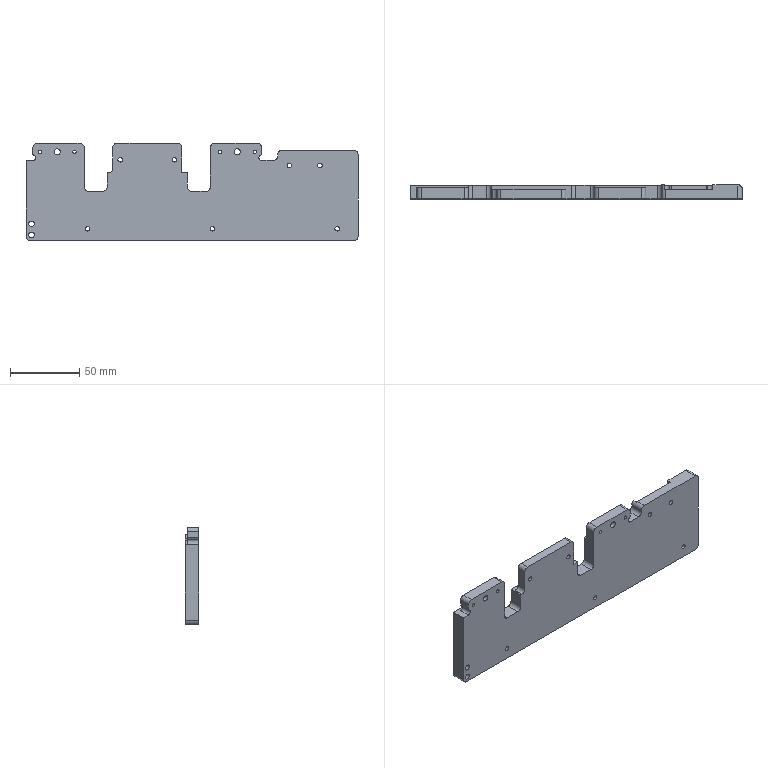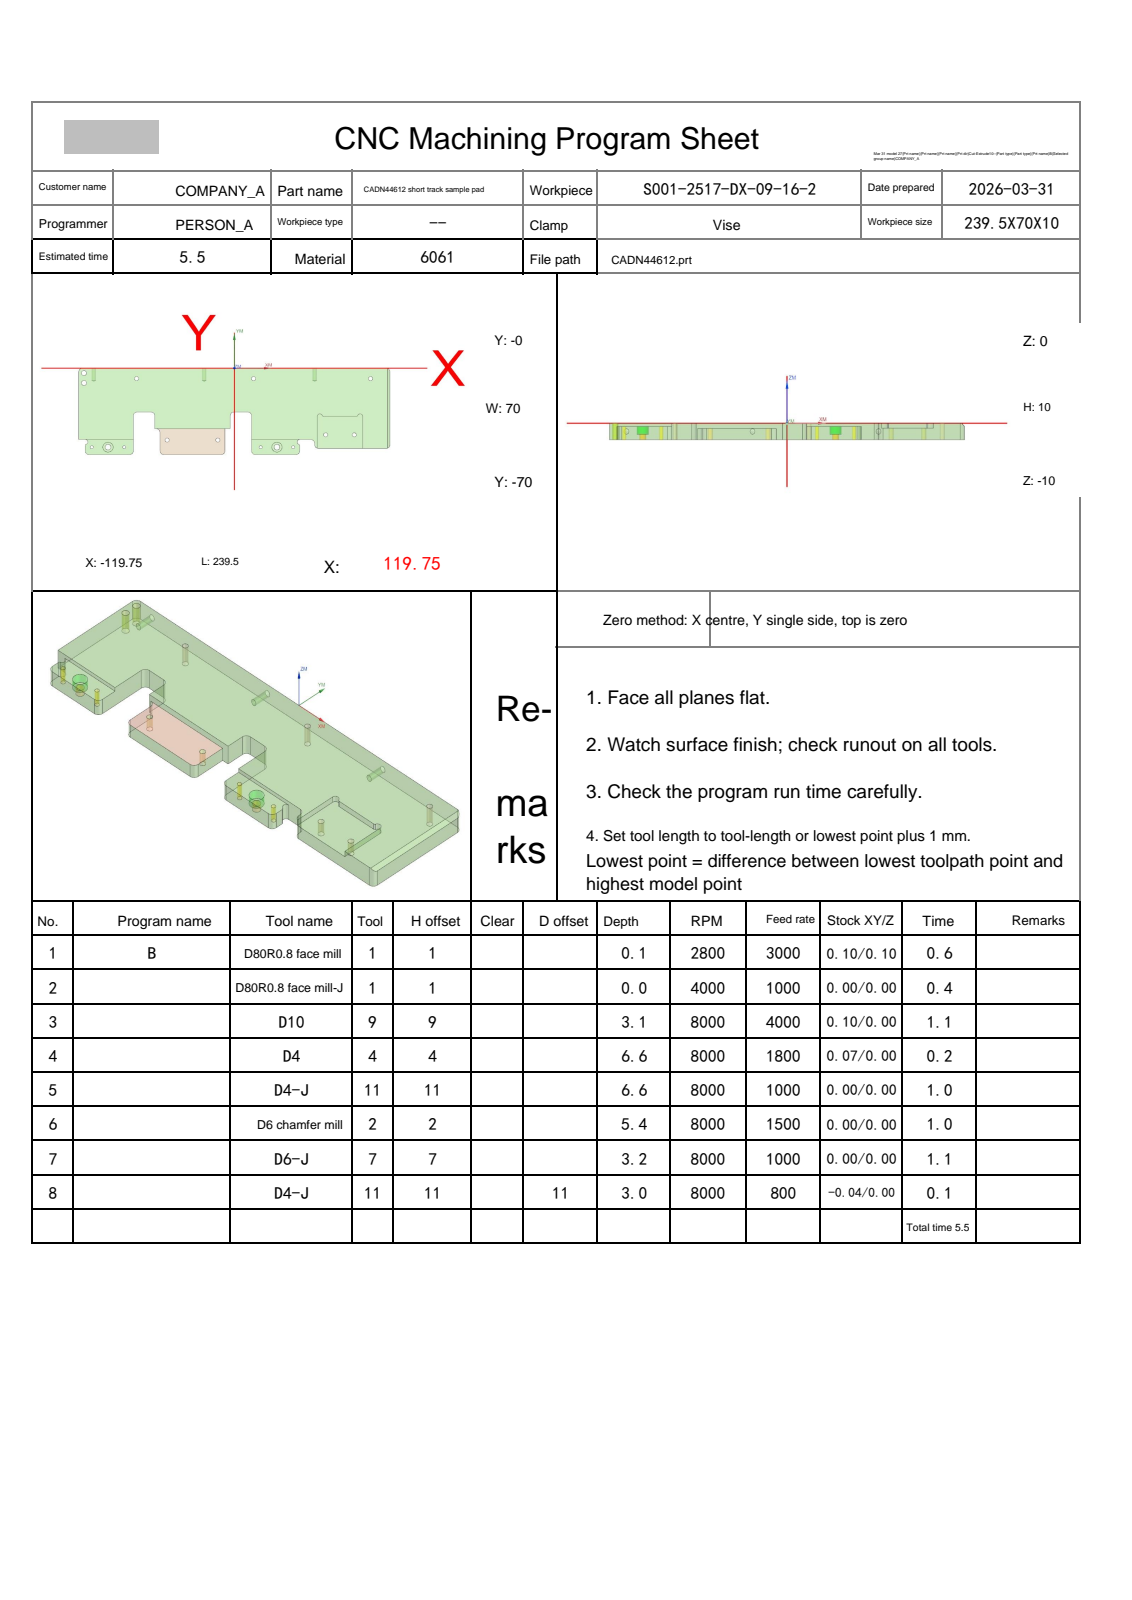NC program | NX | posted by the shop | part box 239.5 x 10 x 70 mm
Whole program, first 1746 of 1845 lines:
%
O0001
(Machine time: 7.06 MIN)
(===Total Tool:6===)
(T1=D80R0.8 face mill D=80.  R=0.8  D-  H01 Z=0.    )
(T9=D10     D=10.  R=0.   D-  H09 Z=-3.1  )
(T4=D4      D=4.   R=0.   D-  H04 Z=-6.6  )
(T11=D4-J   D=4.   R=0.   D-  H11 Z=-6.6  )
(T2=D6 chamfer mill   D=6.   R=0.   D-  H02 Z=-5.4  )
(T7=D6-J    D=6.   R=0.   D7  H07 Z=-3.2  )
G80 G90 G17 G49 G40
G91 G28 Z0
M01
N1 T01 M06
(D80R0.8 face mill  D=80. R=0.8 H=01 ce=0.10 di=0.10)
G00 G90 G54 X-171.847 Y-37.679 M03 S2800
G43 H01 Z20.
M08
Z3.525
G01 Z1.525 F3000.
X-159.847 Y-37.445
X159.847 Y-31.197
X171.847 Y-30.963
Z3.525
G00 X-171.847 Y-37.679
Z3.05
G01 Z1.05
X-159.847 Y-37.445
X159.847 Y-31.197
X171.847 Y-30.963
Z3.05
G00 X-171.847 Y-37.679
Z2.575
G01 Z.575
X-159.847 Y-37.445
X159.847 Y-31.197
X171.847 Y-30.963
Z2.575
G00 X-171.847 Y-37.679
Z2.1
G01 Z.1
X-159.847 Y-37.445
X159.847 Y-31.197
X171.847 Y-30.963
Z2.1
G00 Z20.
G91 G28 Z0.0
M05
M09
G91 G28 Z0.0
M01
N2 T01 M06
(D80R0.8 face mill-J  D=80. R=0.8 H=01 ce=0.00 di=0.00)
G00 G90 G54 X-171.749 Y-37.674 M03 S4000
G43 H01 Z20.
M08
Z2.
G01 Z0.0 F1000.
X-159.749 Y-37.44
X159.749 Y-31.203
X171.749 Y-30.969
Z2.
G00 Z20.
G91 G28 Z0.0
M05
M09
G91 G28 Z0.0
M01
N3 T09 M06
(D10  D=10. R=0. H=09 ce=0.10 di=0.10)
G00 G90 G54 X-122.211 Y-70.4 M03 S8000
G43 H09 Z11.803
M08
Z1.025
G01 Z-.475 F4000.
X-118.881
X-74.28
G03 X-73.343 Y-69.748 I-.001 J1.
X-72.85 Y-67. I-7.407 J2.748
G01 X-71.903 Y-64.223
G03 X-71.85 Y-63.9 I-.947 J.323
X-72.85 Y-62.9 I-1. J0.0
G01 X-119.65
X-127.85
Z1.025
G00 X-122.211 Y-70.4
Z.55
G01 Z-.95
X-118.881
X-74.28
G03 X-73.343 Y-69.748 I-.001 J1.
X-72.85 Y-67. I-7.407 J2.748
G01 X-71.903 Y-64.223
G03 X-71.85 Y-63.9 I-.947 J.323
X-72.85 Y-62.9 I-1. J0.0
G01 X-119.65
X-127.85
Z.55
G00 X-122.211 Y-70.4
Z.075
G01 Z-1.425
X-118.881
X-74.28
G03 X-73.343 Y-69.748 I-.001 J1.
X-72.85 Y-67. I-7.407 J2.748
G01 X-71.903 Y-64.223
G03 X-71.85 Y-63.9 I-.947 J.323
X-72.85 Y-62.9 I-1. J0.0
G01 X-119.65
X-127.85
Z.075
G00 X-122.211 Y-70.4
Z-.4
G01 Z-1.9
X-118.881
X-74.28
G03 X-73.343 Y-69.748 I-.001 J1.
X-72.85 Y-67. I-7.407 J2.748
G01 X-71.903 Y-64.223
G03 X-71.85 Y-63.9 I-.947 J.323
X-72.85 Y-62.9 I-1. J0.0
G01 X-119.65
X-127.85
Z-.4
G00 Z3.
X5.789 Y-70.4
Z1.025
G01 Z-.475
X9.119
X53.72
G03 X54.657 Y-69.748 I-.001 J1.
X55.15 Y-67. I-7.407 J2.748
G01 X56.097 Y-64.223
G03 X56.15 Y-63.9 I-.947 J.323
X55.15 Y-62.9 I-1. J0.0
G01 X8.35
X5.15
Z1.025
G00 X5.789 Y-70.4
Z.55
G01 Z-.95
X9.119
X53.72
G03 X54.657 Y-69.748 I-.001 J1.
X55.15 Y-67. I-7.407 J2.748
G01 X56.097 Y-64.223
G03 X56.15 Y-63.9 I-.947 J.323
X55.15 Y-62.9 I-1. J0.0
G01 X8.35
X5.15
Z.55
G00 X5.789 Y-70.4
Z.075
G01 Z-1.425
X9.119
X53.72
G03 X54.657 Y-69.748 I-.001 J1.
X55.15 Y-67. I-7.407 J2.748
G01 X56.097 Y-64.223
G03 X56.15 Y-63.9 I-.947 J.323
X55.15 Y-62.9 I-1. J0.0
G01 X8.35
X5.15
Z.075
G00 X5.789 Y-70.4
Z-.4
G01 Z-1.9
X9.119
X53.72
G03 X54.657 Y-69.748 I-.001 J1.
X55.15 Y-67. I-7.407 J2.748
G01 X56.097 Y-64.223
G03 X56.15 Y-63.9 I-.947 J.323
X55.15 Y-62.9 I-1. J0.0
G01 X8.35
X5.15
Z-.4
G00 Z11.803
G00 G90 X-62.652 Y-74.1 M03 S8000
Z11.803
Z.983
G01 Z-.517 F4000.
X-57.714
X-7.025
G03 X-6.558 Y-73.984 I-.001 J1.
X-2.91 Y-69.921 I-3.692 J6.984
X-2.868 Y-69.7 I-.558 J.221
X-3.467 Y-69.1 I-.6 J0.0
G01 X-61.062
G02 X-62.049 Y-68.26 I.001 J1.
X-62.15 Y-67. I7.799 J1.26
G01 Y-62.599
G02 X-61.151 Y-61.6 I1. J-.001
G01 X-3.206
G03 X-2.218 Y-60.754 I-.001 J1.
G01 X-1.362 Y-55.254
X-1.35 Y-55.1
G03 X-2.35 Y-54.1 I-1. J0.0
G01 X-62.15
X-69.35
Z.983
G00 X-62.652 Y-74.1
Z.467
G01 Z-1.033
X-57.714
X-7.025
G03 X-6.558 Y-73.984 I-.001 J1.
X-2.91 Y-69.921 I-3.692 J6.984
X-2.868 Y-69.7 I-.558 J.221
X-3.467 Y-69.1 I-.6 J0.0
G01 X-61.062
G02 X-62.049 Y-68.26 I.001 J1.
X-62.15 Y-67. I7.799 J1.26
G01 Y-62.599
G02 X-61.151 Y-61.6 I1. J-.001
G01 X-3.206
G03 X-2.218 Y-60.754 I-.001 J1.
G01 X-1.362 Y-55.254
X-1.35 Y-55.1
G03 X-2.35 Y-54.1 I-1. J0.0
G01 X-62.15
X-69.35
Z.467
G00 X-62.652 Y-74.1
Z-.05
G01 Z-1.55
X-57.714
X-7.025
G03 X-6.558 Y-73.984 I-.001 J1.
X-2.91 Y-69.921 I-3.692 J6.984
X-2.868 Y-69.7 I-.558 J.221
X-3.467 Y-69.1 I-.6 J0.0
G01 X-61.062
G02 X-62.049 Y-68.26 I.001 J1.
X-62.15 Y-67. I7.799 J1.26
G01 Y-62.599
G02 X-61.151 Y-61.6 I1. J-.001
G01 X-3.206
G03 X-2.218 Y-60.754 I-.001 J1.
G01 X-1.362 Y-55.254
X-1.35 Y-55.1
G03 X-2.35 Y-54.1 I-1. J0.0
G01 X-62.15
X-69.35
Z-.05
G00 X-62.652 Y-74.1
Z-.567
G01 Z-2.067
X-57.714
X-7.025
G03 X-6.558 Y-73.984 I-.001 J1.
X-2.91 Y-69.921 I-3.692 J6.984
X-2.868 Y-69.7 I-.558 J.221
X-3.467 Y-69.1 I-.6 J0.0
G01 X-61.062
G02 X-62.049 Y-68.26 I.001 J1.
X-62.15 Y-67. I7.799 J1.26
G01 Y-62.599
G02 X-61.151 Y-61.6 I1. J-.001
G01 X-3.206
G03 X-2.218 Y-60.754 I-.001 J1.
G01 X-1.362 Y-55.254
X-1.35 Y-55.1
G03 X-2.35 Y-54.1 I-1. J0.0
G01 X-62.15
X-69.35
Z-.567
G00 X-62.652 Y-74.1
Z-1.083
G01 Z-2.583
X-57.714
X-7.025
G03 X-6.558 Y-73.984 I-.001 J1.
X-2.91 Y-69.921 I-3.692 J6.984
X-2.868 Y-69.7 I-.558 J.221
X-3.467 Y-69.1 I-.6 J0.0
G01 X-61.062
G02 X-62.049 Y-68.26 I.001 J1.
X-62.15 Y-67. I7.799 J1.26
G01 Y-62.599
G02 X-61.151 Y-61.6 I1. J-.001
G01 X-3.206
G03 X-2.218 Y-60.754 I-.001 J1.
G01 X-1.362 Y-55.254
X-1.35 Y-55.1
G03 X-2.35 Y-54.1 I-1. J0.0
G01 X-62.15
X-69.35
Z-1.083
G00 X-62.652 Y-74.1
Z-1.6
G01 Z-3.1
X-57.714
X-7.025
G03 X-6.558 Y-73.984 I-.001 J1.
X-2.91 Y-69.921 I-3.692 J6.984
X-2.868 Y-69.7 I-.558 J.221
X-3.467 Y-69.1 I-.6 J0.0
G01 X-61.062
G02 X-62.049 Y-68.26 I.001 J1.
X-62.15 Y-67. I7.799 J1.26
G01 Y-62.599
G02 X-61.151 Y-61.6 I1. J-.001
G01 X-3.206
G03 X-2.218 Y-60.754 I-.001 J1.
G01 X-1.362 Y-55.254
X-1.35 Y-55.1
G03 X-2.35 Y-54.1 I-1. J0.0
G01 X-62.15
X-69.35
Z-1.6
G00 Z11.803
G00 G90 X76.35 Y-73. M03 S8000
Z11.803
Z.92
G01 Z-.58 F4000.
Y-69.9
Y-52.598
G02 X77.348 Y-51.6 I1. J-.002
G01 X85.152
G02 X86.15 Y-52.598 I-.002 J-1.
G01 Y-69.044
G03 X86.996 Y-70.032 I1. J0.0
G01 X92.496 Y-70.888
X92.65 Y-70.9
G03 X93.65 Y-69.9 I0.0 J1.
G01 Y-44.1
X68.85
Y-69.9
Y-75.223
Z.92
G00 X76.35 Y-73.
Z.34
G01 Z-1.16
Y-69.9
Y-52.598
G02 X77.348 Y-51.6 I1. J-.002
G01 X85.152
G02 X86.15 Y-52.598 I-.002 J-1.
G01 Y-69.044
G03 X86.996 Y-70.032 I1. J0.0
G01 X92.496 Y-70.888
X92.65 Y-70.9
G03 X93.65 Y-69.9 I0.0 J1.
G01 Y-44.1
X68.85
Y-69.9
Y-75.223
Z.34
G00 X76.35 Y-73.
Z-.24
G01 Z-1.74
Y-69.9
Y-52.598
G02 X77.348 Y-51.6 I1. J-.002
G01 X85.152
G02 X86.15 Y-52.598 I-.002 J-1.
G01 Y-69.044
G03 X86.996 Y-70.032 I1. J0.0
G01 X92.496 Y-70.888
X92.65 Y-70.9
G03 X93.65 Y-69.9 I0.0 J1.
G01 Y-44.1
X68.85
Y-69.9
Y-75.223
Z-.24
G00 X76.35 Y-73.
Z-.82
G01 Z-2.32
Y-69.9
Y-52.598
G02 X77.348 Y-51.6 I1. J-.002
G01 X85.152
G02 X86.15 Y-52.598 I-.002 J-1.
G01 Y-69.044
G03 X86.996 Y-70.032 I1. J0.0
G01 X92.496 Y-70.888
X92.65 Y-70.9
G03 X93.65 Y-69.9 I0.0 J1.
G01 Y-44.1
X68.85
Y-69.9
Y-75.223
Z-.82
G00 X76.35 Y-73.
Z-1.4
G01 Z-2.9
Y-69.9
Y-52.598
G02 X77.348 Y-51.6 I1. J-.002
G01 X85.152
G02 X86.15 Y-52.598 I-.002 J-1.
G01 Y-69.044
G03 X86.996 Y-70.032 I1. J0.0
G01 X92.496 Y-70.888
X92.65 Y-70.9
G03 X93.65 Y-69.9 I0.0 J1.
G01 Y-44.1
X68.85
Y-69.9
Y-75.223
Z-1.4
G00 Z11.803
G00 G90 X122.981 Y9.6 M03 S7000
Z11.8
Z.359
G01 Z-.141 F4000.
X122.99 Y.878
X122.991 Y-.226
Y-65.67
X122.989 Y-65.878
X123.13 Y-65.817 Z-.283
X123.133 Y-65.67
Y-.288
X123.131 Y.817
X123.271 Y.753 Z-.424
X123.274 Y.546
Y-65.67
X123.272 Y-65.755
X123.415 Y-65.693 Z-.566
X123.416 Y-64.562
Y.546
X123.413 Y.69
X123.555 Y.62 Z-.707
X123.557 Y.546
Y-64.471
X123.556 Y-65.616
X123.696 Y-65.529 Z-.849
X123.699 Y-64.366
Y-.634
X123.698 Y.54
X123.839 Y.447 Z-.99
X123.84 Y-.752
Y-65.22
X123.837 Y-65.443
X123.978 Y-65.349 Z-1.131
X123.981 Y-65.22
Y-.887
X123.978 Y.347
X124.119 Y.23 Z-1.273
X124.123 Y.095
Y-63.959
X124.122 Y-65.239
X124.262 Y-65.114 Z-1.414
X124.265 Y-63.869
X124.264 Y-63.78
Y-1.22
X124.263 Y.114
X124.404 Y-.018 Z-1.556
X124.406 Y-1.429
Y-64.77
X124.403 Y-64.983
X124.514 Y-64.864 Z-1.667
X124.517 Y-64.77
X124.518 Y-63.418
X124.517 Y-63.377
Y-.355
X124.514 Y-.143
X124.625 Y-.269 Z-1.778
X124.628 Y-.355
X124.629 Y-1.707
X124.628 Y-1.86
Y-63.14
X124.627 Y-64.741
X124.736 Y-64.597 Z-1.889
X124.739 Y-64.319
Y-2.18
X124.741 Y-2.157
X124.738 Y-.4
X124.843 Y-.544 Z-2.
X124.845 Y-2.829
Y-64.319
X124.842 Y-64.457
G00 Z11.8
G91 G28 Z0.0
M05
M09
G91 G28 Z0.0
M01
N4 T04 M06
(D4  D=4. R=0. H=04 ce=0.07 di=0.00)
G00 G90 G54 X-97.25 Y-64. M03 S8000
G43 H04 Z20.
M08
Z-1.7
G03 X-96.285 Y-64.965 I.965 J0.0 F1800.
X-95.32 Y-64. I0.0 J.965
X-95.32 Y-64. Z-2.05 I-1.93 J0.0
X-95.32 Y-64. Z-2.4 I-1.93 J0.0
X-95.32 Y-64. Z-2.75 I-1.93 J0.0
X-95.32 Y-64. Z-3.1 I-1.93 J0.0
X-95.32 Y-64. Z-3.45 I-1.93 J0.0
X-95.32 Y-64. Z-3.8 I-1.93 J0.0
X-95.32 Y-64. Z-4.15 I-1.93 J0.0
X-95.32 Y-64. Z-4.5 I-1.93 J0.0
X-95.32 Y-64. Z-4.85 I-1.93 J0.0
X-95.32 Y-64. Z-5.2 I-1.93 J0.0
X-95.32 Y-64. Z-5.55 I-1.93 J0.0
X-95.32 Y-64. Z-5.9 I-1.93 J0.0
X-95.32 Y-64. Z-6.25 I-1.93 J0.0
X-95.32 Y-64. Z-6.6 I-1.93 J0.0
X-97.25 Y-62.07 I-1.93 J0.0
X-99.18 Y-64. I0.0 J-1.93
X-97.25 Y-65.93 I1.93 J0.0
X-95.32 Y-64. I0.0 J1.93
X-96.285 Y-63.035 I-.965 J0.0
X-97.25 Y-64. I0.0 J-.965
G00 Z20.
X32.75
Z-1.7
G03 X33.715 Y-64.965 I.965 J0.0
X34.68 Y-64. I0.0 J.965
X34.68 Y-64. Z-2.05 I-1.93 J0.0
X34.68 Y-64. Z-2.4 I-1.93 J0.0
X34.68 Y-64. Z-2.75 I-1.93 J0.0
X34.68 Y-64. Z-3.1 I-1.93 J0.0
X34.68 Y-64. Z-3.45 I-1.93 J0.0
X34.68 Y-64. Z-3.8 I-1.93 J0.0
X34.68 Y-64. Z-4.15 I-1.93 J0.0
X34.68 Y-64. Z-4.5 I-1.93 J0.0
X34.68 Y-64. Z-4.85 I-1.93 J0.0
X34.68 Y-64. Z-5.2 I-1.93 J0.0
X34.68 Y-64. Z-5.55 I-1.93 J0.0
X34.68 Y-64. Z-5.9 I-1.93 J0.0
X34.68 Y-64. Z-6.25 I-1.93 J0.0
X34.68 Y-64. Z-6.6 I-1.93 J0.0
X32.75 Y-62.07 I-1.93 J0.0
X30.82 Y-64. I0.0 J-1.93
X32.75 Y-65.93 I1.93 J0.0
X34.68 Y-64. I0.0 J1.93
X33.715 Y-63.035 I-.965 J0.0
X32.75 Y-64. I0.0 J-.965
G00 Z20.
G91 G28 Z0.0
M05
M09
G91 G28 Z0.0
M01
N5 T11 M06
(D4-J  D=4. R=0. H=11 ce=0.00 di=0.00)
G00 G90 G54 X-97.25 Y-64. M03 S8000
G43 H11 Z20.
M08
Z-6.6
G01 X-95.654 Y-64.329 F600.
X-95.586 Y-64.336
G03 X-95.25 Y-64. I0.0 J.336
X-97.25 Y-62. I-2. J0.0
X-99.25 Y-64. I0.0 J-2.
X-97.25 Y-66. I2. J0.0
X-95.25 Y-64. I0.0 J2.
X-95.312 Y-63.505 I-2. J0.0
X-95.638 Y-63.252 I-.325 J-.083
G01 X-95.785 Y-63.286
X-97.25 Y-64.
G00 Z20.
X32.75
Z-6.6
G01 X34.346 Y-64.329
X34.414 Y-64.336
G03 X34.75 Y-64. I0.0 J.336
X32.75 Y-62. I-2. J0.0
X30.75 Y-64. I0.0 J-2.
X32.75 Y-66. I2. J0.0
X34.75 Y-64. I0.0 J2.
X34.688 Y-63.505 I-2. J0.0
X34.362 Y-63.252 I-.325 J-.083
G01 X34.215 Y-63.286
X32.75 Y-64.
G00 Z20.
G00 G90 X96.341 Y-44.404 M03 S8000
Z20.
Z.15
G01 X96.347 Y-44.403 Z.089 F1000.
X96.361 Y-44.399 Z.034
X96.384 Y-44.393 Z-.014
X96.413 Y-44.384 Z-.058
X96.447 Y-44.371 Z-.096
X96.485 Y-44.355 Z-.129
X96.525 Y-44.335 Z-.157
X96.566 Y-44.311 Z-.181
X96.606 Y-44.282 Z-.201
X96.644 Y-44.249 Z-.217
X96.678 Y-44.211 Z-.23
X96.708 Y-44.168 Z-.239
X96.73 Y-44.119 Z-.245
X96.745 Y-44.064 Z-.249
X96.75 Y-44.003 Z-.25
Y-39.015
Y-39.
G02 X93.922 Y-41. I-2.828 J1.
G01 X93.716
X93.673 Y-41.014 Z-.251
X93.652 Y-41.053 Z-.253
X93.651 Y-41.116 Z-.256
X93.67 Y-41.199 Z-.261
X93.705 Y-41.299 Z-.267
X93.756 Y-41.414 Z-.274
X93.821 Y-41.541 Z-.281
X93.898 Y-41.677 Z-.29
X94.035 Y-41.896 Z-.303
X94.185 Y-42.114 Z-.318
X94.499 Y-42.509 Z-.346
X94.848 Y-42.883 Z-.375
X95.225 Y-43.229 Z-.404
X95.624 Y-43.54 Z-.432
X95.844 Y-43.689 Z-.447
X96.065 Y-43.825 Z-.46
X96.203 Y-43.901 Z-.469
X96.331 Y-43.965 Z-.476
X96.447 Y-44.015 Z-.483
X96.549 Y-44.05 Z-.489
X96.633 Y-44.068 Z-.494
X96.696 Y-44.067 Z-.497
X96.736 Y-44.046 Z-.499
X96.75 Y-44.003 Z-.5
Y-39.015
Y-39.
G02 X93.922 Y-41. I-2.828 J1.
G01 X93.716
X93.673 Y-41.014 Z-.501
X93.652 Y-41.053 Z-.503
X93.651 Y-41.116 Z-.506
X93.67 Y-41.199 Z-.511
X93.705 Y-41.299 Z-.517
X93.756 Y-41.414 Z-.524
X93.821 Y-41.541 Z-.531
X93.898 Y-41.677 Z-.54
X94.035 Y-41.896 Z-.553
X94.185 Y-42.114 Z-.568
X94.499 Y-42.509 Z-.596
X94.848 Y-42.883 Z-.625
X95.225 Y-43.229 Z-.654
X95.624 Y-43.54 Z-.682
X95.844 Y-43.689 Z-.697
X96.065 Y-43.825 Z-.71
X96.203 Y-43.901 Z-.719
X96.331 Y-43.965 Z-.726
X96.447 Y-44.015 Z-.733
X96.549 Y-44.05 Z-.739
X96.633 Y-44.068 Z-.744
X96.696 Y-44.067 Z-.747
X96.736 Y-44.046 Z-.749
X96.75 Y-44.003 Z-.75
Y-39.015
Y-39.
G02 X93.922 Y-41. I-2.828 J1.
G01 X93.716
X93.673 Y-41.014 Z-.751
X93.652 Y-41.053 Z-.753
X93.651 Y-41.116 Z-.756
X93.67 Y-41.199 Z-.761
X93.705 Y-41.299 Z-.767
X93.756 Y-41.414 Z-.774
X93.821 Y-41.541 Z-.781
X93.898 Y-41.677 Z-.79
X94.035 Y-41.896 Z-.803
X94.185 Y-42.114 Z-.818
X94.499 Y-42.509 Z-.846
X94.848 Y-42.883 Z-.875
X95.225 Y-43.229 Z-.904
X95.624 Y-43.54 Z-.932
X95.844 Y-43.689 Z-.947
X96.065 Y-43.825 Z-.96
X96.203 Y-43.901 Z-.969
X96.331 Y-43.965 Z-.976
X96.447 Y-44.015 Z-.983
X96.549 Y-44.05 Z-.989
X96.633 Y-44.068 Z-.994
X96.696 Y-44.067 Z-.997
X96.736 Y-44.046 Z-.999
X96.75 Y-44.003 Z-1.
Y-39.015
Y-39.
G02 X93.922 Y-41. I-2.828 J1.
G01 X93.716
X93.673 Y-41.014 Z-1.001
X93.652 Y-41.053 Z-1.003
X93.651 Y-41.116 Z-1.006
X93.67 Y-41.199 Z-1.011
X93.705 Y-41.299 Z-1.017
X93.756 Y-41.414 Z-1.024
X93.821 Y-41.541 Z-1.031
X93.898 Y-41.677 Z-1.04
X94.035 Y-41.896 Z-1.053
X94.185 Y-42.114 Z-1.068
X94.499 Y-42.509 Z-1.096
X94.848 Y-42.883 Z-1.125
X95.225 Y-43.229 Z-1.154
X95.624 Y-43.54 Z-1.182
X95.844 Y-43.689 Z-1.197
X96.065 Y-43.825 Z-1.21
X96.203 Y-43.901 Z-1.219
X96.331 Y-43.965 Z-1.226
X96.447 Y-44.015 Z-1.233
X96.549 Y-44.05 Z-1.239
X96.633 Y-44.068 Z-1.244
X96.696 Y-44.067 Z-1.247
X96.736 Y-44.046 Z-1.249
X96.75 Y-44.003 Z-1.25
Y-39.015
Y-39.
G02 X93.922 Y-41. I-2.828 J1.
G01 X93.716
X93.673 Y-41.014 Z-1.251
X93.652 Y-41.053 Z-1.253
X93.651 Y-41.116 Z-1.256
X93.67 Y-41.199 Z-1.261
X93.705 Y-41.299 Z-1.267
X93.756 Y-41.414 Z-1.274
X93.821 Y-41.541 Z-1.281
X93.898 Y-41.677 Z-1.29
X94.035 Y-41.896 Z-1.303
X94.185 Y-42.114 Z-1.318
X94.499 Y-42.509 Z-1.346
X94.848 Y-42.883 Z-1.375
X95.225 Y-43.229 Z-1.404
X95.624 Y-43.54 Z-1.432
X95.844 Y-43.689 Z-1.447
X96.065 Y-43.825 Z-1.46
X96.203 Y-43.901 Z-1.469
X96.331 Y-43.965 Z-1.476
X96.447 Y-44.015 Z-1.483
X96.549 Y-44.05 Z-1.489
X96.633 Y-44.068 Z-1.494
X96.696 Y-44.067 Z-1.497
X96.736 Y-44.046 Z-1.499
X96.75 Y-44.003 Z-1.5
Y-39.015
Y-39.
G02 X93.922 Y-41. I-2.828 J1.
G01 X93.716
X93.673 Y-41.014 Z-1.501
X93.652 Y-41.053 Z-1.503
X93.651 Y-41.116 Z-1.506
X93.67 Y-41.199 Z-1.511
X93.705 Y-41.299 Z-1.517
X93.756 Y-41.414 Z-1.524
X93.821 Y-41.541 Z-1.531
X93.898 Y-41.677 Z-1.54
X94.035 Y-41.896 Z-1.553
X94.185 Y-42.114 Z-1.568
X94.499 Y-42.509 Z-1.596
X94.848 Y-42.883 Z-1.625
X95.225 Y-43.229 Z-1.654
X95.624 Y-43.54 Z-1.682
X95.844 Y-43.689 Z-1.697
X96.065 Y-43.825 Z-1.71
X96.203 Y-43.901 Z-1.719
X96.331 Y-43.965 Z-1.726
X96.447 Y-44.015 Z-1.733
X96.549 Y-44.05 Z-1.739
X96.633 Y-44.068 Z-1.744
X96.696 Y-44.067 Z-1.747
X96.736 Y-44.046 Z-1.749
X96.75 Y-44.003 Z-1.75
Y-39.015
Y-39.
G02 X93.922 Y-41. I-2.828 J1.
G01 X93.716
X93.673 Y-41.014 Z-1.751
X93.652 Y-41.053 Z-1.753
X93.651 Y-41.116 Z-1.756
X93.67 Y-41.199 Z-1.761
X93.705 Y-41.299 Z-1.767
X93.756 Y-41.414 Z-1.774
X93.821 Y-41.541 Z-1.781
X93.898 Y-41.677 Z-1.79
X94.035 Y-41.896 Z-1.803
X94.185 Y-42.114 Z-1.818
X94.499 Y-42.509 Z-1.846
X94.848 Y-42.883 Z-1.875
X95.225 Y-43.229 Z-1.904
X95.624 Y-43.54 Z-1.932
X95.844 Y-43.689 Z-1.947
X96.065 Y-43.825 Z-1.96
X96.203 Y-43.901 Z-1.969
X96.331 Y-43.965 Z-1.976
X96.447 Y-44.015 Z-1.983
X96.549 Y-44.05 Z-1.989
X96.633 Y-44.068 Z-1.994
X96.696 Y-44.067 Z-1.997
X96.736 Y-44.046 Z-1.999
X96.75 Y-44.003 Z-2.
Y-39.015
Y-39.
G02 X93.922 Y-41. I-2.828 J1.
G01 X93.716
X93.673 Y-41.014 Z-2.001
X93.652 Y-41.053 Z-2.003
X93.651 Y-41.116 Z-2.006
X93.67 Y-41.199 Z-2.011
X93.705 Y-41.299 Z-2.017
X93.756 Y-41.414 Z-2.024
X93.821 Y-41.541 Z-2.031
X93.898 Y-41.677 Z-2.04
X94.035 Y-41.896 Z-2.053
X94.185 Y-42.114 Z-2.068
X94.499 Y-42.509 Z-2.096
X94.848 Y-42.883 Z-2.125
X95.225 Y-43.229 Z-2.154
X95.624 Y-43.54 Z-2.182
X95.844 Y-43.689 Z-2.197
X96.065 Y-43.825 Z-2.21
X96.203 Y-43.901 Z-2.219
X96.331 Y-43.965 Z-2.226
X96.447 Y-44.015 Z-2.233
X96.549 Y-44.05 Z-2.239
X96.633 Y-44.068 Z-2.244
X96.696 Y-44.067 Z-2.247
X96.736 Y-44.046 Z-2.249
X96.75 Y-44.003 Z-2.25
Y-39.015
Y-39.
G02 X93.922 Y-41. I-2.828 J1.
G01 X93.716
X93.673 Y-41.014 Z-2.251
X93.652 Y-41.053 Z-2.253
X93.651 Y-41.116 Z-2.256
X93.67 Y-41.199 Z-2.261
X93.705 Y-41.299 Z-2.267
X93.756 Y-41.414 Z-2.274
X93.821 Y-41.541 Z-2.281
X93.898 Y-41.677 Z-2.29
X94.035 Y-41.896 Z-2.303
X94.185 Y-42.114 Z-2.318
X94.499 Y-42.509 Z-2.346
X94.848 Y-42.883 Z-2.375
X95.225 Y-43.229 Z-2.404
X95.624 Y-43.54 Z-2.432
X95.844 Y-43.689 Z-2.447
X96.065 Y-43.825 Z-2.46
X96.203 Y-43.901 Z-2.469
X96.331 Y-43.965 Z-2.476
X96.447 Y-44.015 Z-2.483
X96.549 Y-44.05 Z-2.489
X96.633 Y-44.068 Z-2.494
X96.696 Y-44.067 Z-2.497
X96.736 Y-44.046 Z-2.499
X96.75 Y-44.003 Z-2.5
Y-39.015
Y-39.
G02 X93.922 Y-41. I-2.828 J1.
G01 X93.716
X93.673 Y-41.014 Z-2.501
X93.652 Y-41.053 Z-2.503
X93.651 Y-41.116 Z-2.506
X93.67 Y-41.199 Z-2.511
X93.705 Y-41.299 Z-2.517
X93.756 Y-41.414 Z-2.524
X93.821 Y-41.541 Z-2.531
X93.898 Y-41.677 Z-2.54
X94.035 Y-41.896 Z-2.553
X94.185 Y-42.114 Z-2.568
X94.499 Y-42.509 Z-2.596
X94.848 Y-42.883 Z-2.625
X95.225 Y-43.229 Z-2.654
X95.624 Y-43.54 Z-2.682
X95.844 Y-43.689 Z-2.697
X96.065 Y-43.825 Z-2.71
X96.203 Y-43.901 Z-2.719
X96.331 Y-43.965 Z-2.726
X96.447 Y-44.015 Z-2.733
X96.549 Y-44.05 Z-2.739
X96.633 Y-44.068 Z-2.744
X96.696 Y-44.067 Z-2.747
X96.736 Y-44.046 Z-2.749
X96.75 Y-44.003 Z-2.75
Y-39.015
Y-39.
G02 X93.922 Y-41. I-2.828 J1.
G01 X93.716
X93.673 Y-41.014 Z-2.751
X93.652 Y-41.053 Z-2.753
X93.651 Y-41.116 Z-2.756
X93.67 Y-41.199 Z-2.761
X93.705 Y-41.299 Z-2.767
X93.756 Y-41.414 Z-2.774
X93.821 Y-41.541 Z-2.781
X93.898 Y-41.677 Z-2.79
X94.035 Y-41.896 Z-2.803
X94.185 Y-42.114 Z-2.818
X94.499 Y-42.509 Z-2.846
X94.848 Y-42.883 Z-2.875
X95.225 Y-43.229 Z-2.904
X95.624 Y-43.54 Z-2.932
X95.844 Y-43.689 Z-2.947
X96.065 Y-43.825 Z-2.96
X96.203 Y-43.901 Z-2.969
X96.331 Y-43.965 Z-2.976
X96.447 Y-44.015 Z-2.983
X96.549 Y-44.05 Z-2.989
X96.633 Y-44.068 Z-2.994
X96.696 Y-44.067 Z-2.997
X96.736 Y-44.046 Z-2.999
X96.75 Y-44.003 Z-3.
Y-39.015
Y-39.
G02 X93.922 Y-41. I-2.828 J1.
G01 X93.716
X93.655 Y-41.005 Z-2.999
X93.6 Y-41.019 Z-2.995
X93.551 Y-41.042 Z-2.989
X93.508 Y-41.07 Z-2.98
X93.47 Y-41.104 Z-2.967
X93.437 Y-41.141 Z-2.951
X93.408 Y-41.18 Z-2.931
X93.384 Y-41.22 Z-2.907
X93.364 Y-41.259 Z-2.879
X93.348 Y-41.296 Z-2.846
X93.336 Y-41.33 Z-2.808
X93.327 Y-41.358 Z-2.764
X93.32 Y-41.381 Z-2.716
X93.317 Y-41.395 Z-2.661
X93.316 Y-41.4 Z-2.6
G00 Z3.
X69.184
Z.15
G01 X69.183 Y-41.395 Z.089
X69.18 Y-41.381 Z.034
X69.173 Y-41.358 Z-.014
X69.164 Y-41.33 Z-.058
X69.152 Y-41.296 Z-.096
X69.136 Y-41.259 Z-.129
X69.116 Y-41.22 Z-.157
X69.092 Y-41.18 Z-.181
X69.063 Y-41.141 Z-.201
X69.03 Y-41.104 Z-.217
X68.992 Y-41.07 Z-.23
X68.949 Y-41.042 Z-.239
X68.9 Y-41.019 Z-.245
X68.845 Y-41.005 Z-.249
X68.784 Y-41. Z-.25
X68.578
G02 X65.75 Y-39. I0.0 J3.
G01 Y-44.003
X65.764 Y-44.046 Z-.251
X65.804 Y-44.067 Z-.253
X65.867 Y-44.068 Z-.256
X65.95 Y-44.05 Z-.261
X66.051 Y-44.015 Z-.267
X66.167 Y-43.965 Z-.274
X66.295 Y-43.901 Z-.281
X66.432 Y-43.825 Z-.29
X66.652 Y-43.688 Z-.303
X66.872 Y-43.54 Z-.318
X67.271 Y-43.229 Z-.346
X67.648 Y-42.883 Z-.375
X67.998 Y-42.509 Z-.404
X68.313 Y-42.113 Z-.432
X68.463 Y-41.896 Z-.447
X68.601 Y-41.677 Z-.46
X68.678 Y-41.541 Z-.469
X68.743 Y-41.414 Z-.476
X68.794 Y-41.299 Z-.483
X68.83 Y-41.199 Z-.489
X68.848 Y-41.116 Z-.494
Y-41.053 Z-.497
X68.827 Y-41.014 Z-.499
X68.784 Y-41. Z-.5
X68.578
G02 X65.75 Y-39. I0.0 J3.
G01 Y-44.003
X65.764 Y-44.046 Z-.501
X65.804 Y-44.067 Z-.503
X65.867 Y-44.068 Z-.506
X65.95 Y-44.05 Z-.511
X66.051 Y-44.015 Z-.517
X66.167 Y-43.965 Z-.524
X66.295 Y-43.901 Z-.531
X66.432 Y-43.825 Z-.54
X66.652 Y-43.688 Z-.553
X66.872 Y-43.54 Z-.568
X67.271 Y-43.229 Z-.596
X67.648 Y-42.883 Z-.625
X67.998 Y-42.509 Z-.654
X68.313 Y-42.113 Z-.682
X68.463 Y-41.896 Z-.697
X68.601 Y-41.677 Z-.71
X68.678 Y-41.541 Z-.719
X68.743 Y-41.414 Z-.726
X68.794 Y-41.299 Z-.733
X68.83 Y-41.199 Z-.739
X68.848 Y-41.116 Z-.744
Y-41.053 Z-.747
X68.827 Y-41.014 Z-.749
X68.784 Y-41. Z-.75
X68.578
G02 X65.75 Y-39. I0.0 J3.
G01 Y-44.003
X65.764 Y-44.046 Z-.751
X65.804 Y-44.067 Z-.753
X65.867 Y-44.068 Z-.756
X65.95 Y-44.05 Z-.761
X66.051 Y-44.015 Z-.767
X66.167 Y-43.965 Z-.774
X66.295 Y-43.901 Z-.781
X66.432 Y-43.825 Z-.79
X66.652 Y-43.688 Z-.803
X66.872 Y-43.54 Z-.818
X67.271 Y-43.229 Z-.846
X67.648 Y-42.883 Z-.875
X67.998 Y-42.509 Z-.904
X68.313 Y-42.113 Z-.932
X68.463 Y-41.896 Z-.947
X68.601 Y-41.677 Z-.96
X68.678 Y-41.541 Z-.969
X68.743 Y-41.414 Z-.976
X68.794 Y-41.299 Z-.983
X68.83 Y-41.199 Z-.989
X68.848 Y-41.116 Z-.994
Y-41.053 Z-.997
X68.827 Y-41.014 Z-.999
X68.784 Y-41. Z-1.
X68.578
G02 X65.75 Y-39. I0.0 J3.
G01 Y-44.003
X65.764 Y-44.046 Z-1.001
X65.804 Y-44.067 Z-1.003
X65.867 Y-44.068 Z-1.006
X65.95 Y-44.05 Z-1.011
X66.051 Y-44.015 Z-1.017
X66.167 Y-43.965 Z-1.024
X66.295 Y-43.901 Z-1.031
X66.432 Y-43.825 Z-1.04
X66.652 Y-43.688 Z-1.053
X66.872 Y-43.54 Z-1.068
X67.271 Y-43.229 Z-1.096
X67.648 Y-42.883 Z-1.125
X67.998 Y-42.509 Z-1.154
X68.313 Y-42.113 Z-1.182
X68.463 Y-41.896 Z-1.197
X68.601 Y-41.677 Z-1.21
X68.678 Y-41.541 Z-1.219
X68.743 Y-41.414 Z-1.226
X68.794 Y-41.299 Z-1.233
X68.83 Y-41.199 Z-1.239
X68.848 Y-41.116 Z-1.244
Y-41.053 Z-1.247
X68.827 Y-41.014 Z-1.249
X68.784 Y-41. Z-1.25
X68.578
G02 X65.75 Y-39. I0.0 J3.
G01 Y-44.003
X65.764 Y-44.046 Z-1.251
X65.804 Y-44.067 Z-1.253
X65.867 Y-44.068 Z-1.256
X65.95 Y-44.05 Z-1.261
X66.051 Y-44.015 Z-1.267
X66.167 Y-43.965 Z-1.274
X66.295 Y-43.901 Z-1.281
X66.432 Y-43.825 Z-1.29
X66.652 Y-43.688 Z-1.303
X66.872 Y-43.54 Z-1.318
X67.271 Y-43.229 Z-1.346
X67.648 Y-42.883 Z-1.375
X67.998 Y-42.509 Z-1.404
X68.313 Y-42.113 Z-1.432
X68.463 Y-41.896 Z-1.447
X68.601 Y-41.677 Z-1.46
X68.678 Y-41.541 Z-1.469
X68.743 Y-41.414 Z-1.476
X68.794 Y-41.299 Z-1.483
X68.83 Y-41.199 Z-1.489
X68.848 Y-41.116 Z-1.494
Y-41.053 Z-1.497
X68.827 Y-41.014 Z-1.499
X68.784 Y-41. Z-1.5
X68.578
G02 X65.75 Y-39. I0.0 J3.
G01 Y-44.003
X65.764 Y-44.046 Z-1.501
X65.804 Y-44.067 Z-1.503
X65.867 Y-44.068 Z-1.506
X65.95 Y-44.05 Z-1.511
X66.051 Y-44.015 Z-1.517
X66.167 Y-43.965 Z-1.524
X66.295 Y-43.901 Z-1.531
X66.432 Y-43.825 Z-1.54
X66.652 Y-43.688 Z-1.553
X66.872 Y-43.54 Z-1.568
X67.271 Y-43.229 Z-1.596
X67.648 Y-42.883 Z-1.625
X67.998 Y-42.509 Z-1.654
X68.313 Y-42.113 Z-1.682
X68.463 Y-41.896 Z-1.697
X68.601 Y-41.677 Z-1.71
X68.678 Y-41.541 Z-1.719
X68.743 Y-41.414 Z-1.726
X68.794 Y-41.299 Z-1.733
X68.83 Y-41.199 Z-1.739
X68.848 Y-41.116 Z-1.744
Y-41.053 Z-1.747
X68.827 Y-41.014 Z-1.749
X68.784 Y-41. Z-1.75
X68.578
G02 X65.75 Y-39. I0.0 J3.
G01 Y-44.003
X65.764 Y-44.046 Z-1.751
X65.804 Y-44.067 Z-1.753
X65.867 Y-44.068 Z-1.756
X65.95 Y-44.05 Z-1.761
X66.051 Y-44.015 Z-1.767
X66.167 Y-43.965 Z-1.774
X66.295 Y-43.901 Z-1.781
X66.432 Y-43.825 Z-1.79
X66.652 Y-43.688 Z-1.803
X66.872 Y-43.54 Z-1.818
X67.271 Y-43.229 Z-1.846
X67.648 Y-42.883 Z-1.875
X67.998 Y-42.509 Z-1.904
X68.313 Y-42.113 Z-1.932
X68.463 Y-41.896 Z-1.947
X68.601 Y-41.677 Z-1.96
X68.678 Y-41.541 Z-1.969
X68.743 Y-41.414 Z-1.976
X68.794 Y-41.299 Z-1.983
X68.83 Y-41.199 Z-1.989
X68.848 Y-41.116 Z-1.994
Y-41.053 Z-1.997
X68.827 Y-41.014 Z-1.999
X68.784 Y-41. Z-2.
X68.578
G02 X65.75 Y-39. I0.0 J3.
G01 Y-44.003
X65.764 Y-44.046 Z-2.001
X65.804 Y-44.067 Z-2.003
X65.867 Y-44.068 Z-2.006
X65.95 Y-44.05 Z-2.011
X66.051 Y-44.015 Z-2.017
X66.167 Y-43.965 Z-2.024
X66.295 Y-43.901 Z-2.031
X66.432 Y-43.825 Z-2.04
X66.652 Y-43.688 Z-2.053
X66.872 Y-43.54 Z-2.068
X67.271 Y-43.229 Z-2.096
X67.648 Y-42.883 Z-2.125
X67.998 Y-42.509 Z-2.154
X68.313 Y-42.113 Z-2.182
X68.463 Y-41.896 Z-2.197
X68.601 Y-41.677 Z-2.21
X68.678 Y-41.541 Z-2.219
X68.743 Y-41.414 Z-2.226
X68.794 Y-41.299 Z-2.233
X68.83 Y-41.199 Z-2.239
X68.848 Y-41.116 Z-2.244
Y-41.053 Z-2.247
X68.827 Y-41.014 Z-2.249
X68.784 Y-41. Z-2.25
X68.578
G02 X65.75 Y-39. I0.0 J3.
G01 Y-44.003
X65.764 Y-44.046 Z-2.251
X65.804 Y-44.067 Z-2.253
X65.867 Y-44.068 Z-2.256
X65.95 Y-44.05 Z-2.261
X66.051 Y-44.015 Z-2.267
X66.167 Y-43.965 Z-2.274
X66.295 Y-43.901 Z-2.281
X66.432 Y-43.825 Z-2.29
X66.652 Y-43.688 Z-2.303
X66.872 Y-43.54 Z-2.318
X67.271 Y-43.229 Z-2.346
X67.648 Y-42.883 Z-2.375
X67.998 Y-42.509 Z-2.404
X68.313 Y-42.113 Z-2.432
X68.463 Y-41.896 Z-2.447
X68.601 Y-41.677 Z-2.46
X68.678 Y-41.541 Z-2.469
X68.743 Y-41.414 Z-2.476
X68.794 Y-41.299 Z-2.483
X68.83 Y-41.199 Z-2.489
X68.848 Y-41.116 Z-2.494
Y-41.053 Z-2.497
X68.827 Y-41.014 Z-2.499
X68.784 Y-41. Z-2.5
X68.578
G02 X65.75 Y-39. I0.0 J3.
G01 Y-44.003
X65.764 Y-44.046 Z-2.501
X65.804 Y-44.067 Z-2.503
X65.867 Y-44.068 Z-2.506
X65.95 Y-44.05 Z-2.511
X66.051 Y-44.015 Z-2.517
X66.167 Y-43.965 Z-2.524
X66.295 Y-43.901 Z-2.531
X66.432 Y-43.825 Z-2.54
X66.652 Y-43.688 Z-2.553
X66.872 Y-43.54 Z-2.568
X67.271 Y-43.229 Z-2.596
X67.648 Y-42.883 Z-2.625
X67.998 Y-42.509 Z-2.654
X68.313 Y-42.113 Z-2.682
X68.463 Y-41.896 Z-2.697
X68.601 Y-41.677 Z-2.71
X68.678 Y-41.541 Z-2.719
X68.743 Y-41.414 Z-2.726
X68.794 Y-41.299 Z-2.733
X68.83 Y-41.199 Z-2.739
X68.848 Y-41.116 Z-2.744
Y-41.053 Z-2.747
X68.827 Y-41.014 Z-2.749
X68.784 Y-41. Z-2.75
X68.578
G02 X65.75 Y-39. I0.0 J3.
G01 Y-44.003
X65.764 Y-44.046 Z-2.751
X65.804 Y-44.067 Z-2.753
X65.867 Y-44.068 Z-2.756
X65.95 Y-44.05 Z-2.761
X66.051 Y-44.015 Z-2.767
X66.167 Y-43.965 Z-2.774
X66.295 Y-43.901 Z-2.781
X66.432 Y-43.825 Z-2.79
X66.652 Y-43.688 Z-2.803
X66.872 Y-43.54 Z-2.818
X67.271 Y-43.229 Z-2.846
X67.648 Y-42.883 Z-2.875
X67.998 Y-42.509 Z-2.904
X68.313 Y-42.113 Z-2.932
X68.463 Y-41.896 Z-2.947
X68.601 Y-41.677 Z-2.96
X68.678 Y-41.541 Z-2.969
X68.743 Y-41.414 Z-2.976
X68.794 Y-41.299 Z-2.983
X68.83 Y-41.199 Z-2.989
X68.848 Y-41.116 Z-2.994
Y-41.053 Z-2.997
X68.827 Y-41.014 Z-2.999
X68.784 Y-41. Z-3.
X68.578
G02 X65.75 Y-39. I0.0 J3.
G01 Y-44.003
X65.755 Y-44.064 Z-2.999
X65.769 Y-44.119 Z-2.995
X65.792 Y-44.167 Z-2.989
X65.82 Y-44.211 Z-2.98
X65.854 Y-44.249 Z-2.967
X65.891 Y-44.282 Z-2.951
X65.93 Y-44.31 Z-2.931
X65.97 Y-44.334 Z-2.907
X66.009 Y-44.354 Z-2.879
X66.046 Y-44.37 Z-2.846
X66.08 Y-44.383 Z-2.808
X66.108 Y-44.392 Z-2.764
X66.131 Y-44.398 Z-2.716
X66.145 Y-44.402 Z-2.661
X66.15 Y-44.403 Z-2.6
G00 Z20.
G00 G90 X82.05 Y-67.8 M03 S8000
Z11.803
Z-1.5
G01 Z-3. F800.
Y-66.2
G03 X81.25 Y-65.4 I-.8 J0.0
G01 X66.549
G02 X66.15 Y-65.001 I.001 J.4
G01 Y-40.568
X66.166 Y-40.505
X66.227 Y-40.478
X66.284 Y-40.509
G03 X68.578 Y-41.4 I2.295 J2.509
G01 X93.922
G03 X96.216 Y-40.509 I0.0 J3.4
G01 X96.273 Y-40.478
X96.334 Y-40.505
X96.35 Y-40.568
Y-65.001
G02 X95.951 Y-65.4 I-.4 J.001
G01 X80.415
G02 X80.133 Y-65.283 I0.0 J.4
G01 X78.367 Y-63.517
G03 X78.085 Y-63.4 I-.283 J-.283
G01 X68.549
G02 X68.15 Y-63.001 I.001 J.4
G01 Y-43.799
G02 X68.551 Y-43.399 I.401 J-.001
G01 X68.578 Y-43.4
X93.949
G02 X94.35 Y-43.799 I0.0 J-.4
G01 Y-63.001
G02 X93.951 Y-63.4 I-.4 J.001
G01 X80.415
G02 X80.133 Y-63.283 I0.0 J.4
G01 X78.367 Y-61.517
G03 X78.085 Y-61.4 I-.283 J-.283
G01 X70.549
G02 X70.15 Y-61.001 I.001 J.4
G01 Y-45.799
G02 X70.549 Y-45.4 I.4 J-.001
G01 X91.951
G02 X92.35 Y-45.799 I-.001 J-.4
G01 Y-61.001
G02 X91.951 Y-61.4 I-.4 J.001
G01 X80.415
G02 X80.133 Y-61.283 I0.0 J.4
G01 X78.367 Y-59.517
G03 X78.084 Y-59.4 I-.283 J-.283
G01 X72.549
G02 X72.15 Y-59.001 I.001 J.4
G01 Y-47.799
G02 X72.549 Y-47.4 I.4 J-.001
G01 X89.951
G02 X90.35 Y-47.799 I-.001 J-.4
G01 Y-59.001
G02 X89.951 Y-59.4 I-.4 J.001
G01 X80.415
G02 X80.133 Y-59.283 I0.0 J.4
G01 X78.367 Y-57.517
G03 X78.084 Y-57.4 I-.283 J-.283
G01 X74.549
G02 X74.15 Y-57.001 I.001 J.4
G01 Y-49.799
G02 X74.549 Y-49.4 I.4 J-.001
G01 X87.951
G02 X88.35 Y-49.799 I-.001 J-.4
G01 Y-57.001
G02 X87.951 Y-57.4 I-.4 J.001
G01 X80.415
G02 X80.133 Y-57.283 I0.0 J.4
G01 X78.367 Y-55.517
G03 X78.084 Y-55.4 I-.283 J-.283
G01 X76.549
G02 X76.15 Y-55.001 I.001 J.4
G01 Y-51.799
G02 X76.549 Y-51.4 I.4 J-.001
G01 X85.951
G02 X86.35 Y-51.799 I-.001 J-.4
G01 Y-55.001
G02 X85.951 Y-55.4 I-.4 J.001
G01 X80.315
G02 X80.033 Y-55.283 I0.0 J.4
G01 X78.467 Y-53.717
G03 X78.184 Y-53.6 I-.283 J-.283
G01 X78.149
G02 X77.95 Y-53.4 I.001 J.2
X78.149 Y-53.2 I.2 J0.0
G01 X84.351
G02 X84.55 Y-53.4 I-.001 J-.2
X84.351 Y-53.6 I-.2 J0.0
G01 X79.25
X78.25
G03 X77.45 Y-54.4 I0.0 J-.8
G01 Z-1.5
G00 Z11.803
G91 G28 Z0.0
M05
M09
G91 G28 Z0.0
M01
N6 T02 M06
(D6 chamfer mill  D=6. R=0. H=02 ce=0.00 di=0.00)
G00 G90 G54 X45.25 Y-64. M03 S8000
G43 H02 Z20.
M08
G98 G81 X45.25 Y-64. Z-3.75 R1. F1000.
X20.25
X-84.75
X-109.75
G80
G00 Z20.
G00 G90 X-75.25 Y-8.5 M03 S8000
Z20.
G98 G81 X-75.25 Y-8.5 Z-2.2 R3. F1000.
X-51.75 Y-58.25 Z-5.4 R-.2
X-12.75
X14.75 Y-8.5 Z-2.2 R3.
X70.25 Y-54. Z-5.2 R0.0
X92.25
X104.75 Y-8.5 Z-2.2 R3.
G80
G00 Z20.
G00 G90 X-115.75 Y-4. M03 S8000
Z20.
G98 G81 X-115.75 Y-4. Z-2.3 R3. F1000.
Y-12.
G80
G00 Z20.
G00 G90 X118.466 Y-65.522 M03 S6500
Z20.
Z2.8
G01 Z-1.2 F1500.
X118.303 Y-65.662
X118.083 Y-65.771
X117.648 Y-65.898
X117.202 Y-65.974
X116.75 Y-66.
X98.75
G02 X97.75 Y-65. I0.0 J1.
G01 Y-39.
G03 X96.75 Y-38. I-1. J0.0
X96.369 Y-38.075 I0.0 J-1.
G01 X96.129 Y-38.217
X95.936 Y-38.419
X95.807 Y-38.667
G02 X93.922 Y-40. I-1.886 J.667
G01 X68.578
G02 X66.693 Y-38.667 I0.0 J2.
G03 X65.75 Y-38. I-.943 J-.333
X65.083 Y-38.255 I0.0 J-1.
G01 X64.903 Y-38.469
X64.789 Y-38.723
X64.75 Y-39.
Y-64.828
G02 X63.75 Y-65.828 I-1. J0.0
X63.417 Y-65.771 I0.0 J1.
X60.75 Y-62. I1.333 J3.771
G01 Y-60.8
G03 X58.75 Y-58.8 I-2. J0.0
G01 X13.25
G02 X12.25 Y-57.8 I0.0 J1.
G01 Y-38.5
G03 X10.25 Y-36.5 I-2. J0.0
G01 X-.25
G03 X-2.25 Y-38.5 I0.0 J-2.
G01 Y-49.
G02 X-3.25 Y-50. I-1. J0.0
G01 X-61.25
G02 X-62.25 Y-49. I0.0 J1.
G01 Y-38.5
G03 X-64.25 Y-36.5 I-2. J0.0
G01 X-74.75
G03 X-76.75 Y-38.5 I0.0 J-2.
G01 Y-57.8
G02 X-77.75 Y-58.8 I-1. J0.0
G01 X-119.75
G02 X-120.75 Y-57.8 I0.0 J1.
G01 Y-3.
G02 X-116.75 Y1. I4. J0.0
G01 X0.0
X116.75
X117.202 Y.974
X117.648 Y.898
X118.083 Y.771
X118.303 Y.662
X118.466 Y.522
Z2.8
G00 Z10.
X104.331 Y-8.994
Z.405
G01 Z-1.2
G03 X104.647 Y-9.141 I1. J1.732
G01 X104.697 Y-9.162
X104.75 Y-9.15
G03 X105.4 Y-8.5 I0.0 J.65
X104.75 Y-7.85 I-.65 J0.0
X104.1 Y-8.5 I0.0 J-.65
X104.75 Y-9.15 I.65 J0.0
G01 X104.803 Y-9.162
X104.853 Y-9.141
G03 X105.169 Y-8.994 I-.684 J1.879
G01 Z.405
G00 Z10.
X14.331
Z.405
G01 Z-1.2
G03 X14.647 Y-9.141 I1. J1.732
G01 X14.697 Y-9.162
X14.75 Y-9.15
G03 X15.4 Y-8.5 I0.0 J.65
X14.75 Y-7.85 I-.65 J0.0
X14.1 Y-8.5 I0.0 J-.65
X14.75 Y-9.15 I.65 J0.0
G01 X14.803 Y-9.162
X14.853 Y-9.141
G03 X15.169 Y-8.994 I-.684 J1.879
G01 Z.405
G00 Z10.
X-75.669
Z.405
G01 Z-1.2
G03 X-75.353 Y-9.141 I1. J1.732
G01 X-75.303 Y-9.162
X-75.25 Y-9.15
G03 X-74.6 Y-8.5 I0.0 J.65
X-75.25 Y-7.85 I-.65 J0.0
X-75.9 Y-8.5 I0.0 J-.65
X-75.25 Y-9.15 I.65 J0.0
G01 X-75.197 Y-9.162
X-75.147 Y-9.141
G03 X-74.831 Y-8.994 I-.684 J1.879
G01 Z.405
G00 Z10.
X-116.162 Y-12.826
Z.33
G01 Z-1.2
G03 X-115.853 Y-12.986 I1.075 J1.687
G01 X-115.804 Y-13.01
X-115.75 Y-13.
G03 X-114.75 Y-12. I0.0 J1.
X-115.75 Y-11. I-1. J0.0
X-116.75 Y-12. I0.0 J-1.
X-115.75 Y-13. I1. J0.0
G01 X-115.696 Y-13.01
X-115.647 Y-12.986
G03 X-115.338 Y-12.826 I-.765 J1.848
G01 Z.33
G00 Z2.55
X-116.162 Y-4.826
Z.33
G01 Z-1.2
G03 X-115.853 Y-4.986 I1.075 J1.687
G01 X-115.804 Y-5.01
X-115.75 Y-5.
G03 X-114.75 Y-4. I0.0 J1.
X-115.75 Y-3. I-1. J0.0
X-116.75 Y-4. I0.0 J-1.
X-115.75 Y-5. I1. J0.0
G01 X-115.696 Y-5.01
X-115.647 Y-4.986
G03 X-115.338 Y-4.826 I-.765 J1.848
G01 Z.33
G00 Z10.
X-76.682 Y-60.775
Z-1.669
G01 Z-3.2
X-76.742 Y-60.861
X-76.75 Y-60.891
Y-67.
G02 X-80.75 Y-71. I-4. J0.0
G01 X-111.75
G02 X-115.75 Y-67. I0.0 J4.
G01 Y-62.628
Y-62.623
G02 X-114.989 Y-61.063 I1.98 J0.0
G01 X-114.976 Y-61.047
X-114.952 Y-60.982
Z-1.642
G00 Z10.
X-97.332 Y-61.174
Z-1.772
G01 Z-3.2
G03 X-97.657 Y-61.048 I-.882 J-1.795
G01 X-97.708 Y-61.03
X-97.761 Y-61.046
X-98.2 Y-61.154
G03 X-100.25 Y-64. I.95 J-2.846
X-97.25 Y-67. I3. J0.0
X-94.25 Y-64. I0.0 J3.
X-96.3 Y-61.154 I-3. J0.0
G01 X-96.739 Y-61.046
X-96.792 Y-61.03
X-96.843 Y-61.048
G03 X-97.168 Y-61.174 I.556 J-1.921
G01 Z-1.772
G00 Z10.
X50.452 Y-60.982
Z-1.642
G01 Z-3.2
X50.476 Y-61.047
X50.489 Y-61.063
X50.525 Y-61.088
G02 X51.25 Y-62.628 I-1.275 J-1.541
G01 Y-67.
G02 X47.25 Y-71. I-4. J0.0
G01 X16.25
G02 X12.25 Y-67. I0.0 J4.
G01 Y-60.891
X12.242 Y-60.861
X12.182 Y-60.775
Z-1.669
G00 Z10.
X32.668 Y-61.174
Z-1.772
G01 Z-3.2
G03 X32.343 Y-61.048 I-.882 J-1.795
G01 X32.292 Y-61.03
X32.239 Y-61.046
X31.8 Y-61.154
G03 X29.75 Y-64. I.95 J-2.846
X32.75 Y-67. I3. J0.0
X35.75 Y-64. I0.0 J3.
X33.7 Y-61.154 I-3. J0.0
G01 X33.261 Y-61.046
X33.208 Y-61.03
X33.157 Y-61.048
G03 X32.832 Y-61.174 I.556 J-1.921
G01 Z-1.772
G00 Z10.
X95.706 Y-66.045
Z-1.82
G01 Z-4.2
X95.649 Y-66.005
X95.629 Y-66.
X66.809
X66.779 Y-66.008
X66.693 Y-66.068
Z-1.795
G00 Z10.
X91.831 Y-54.494
Z-2.595
G01 Z-4.2
G03 X92.147 Y-54.641 I1. J1.732
G01 X92.197 Y-54.662
X92.25 Y-54.65
G03 X92.9 Y-54. I0.0 J.65
X92.25 Y-53.35 I-.65 J0.0
X91.6 Y-54. I0.0 J-.65
X92.25 Y-54.65 I.65 J0.0
G01 X92.303 Y-54.662
X92.353 Y-54.641
G03 X92.669 Y-54.494 I-.684 J1.879
G01 Z-2.595
G00 Z10.
X69.831
Z-2.595
G01 Z-4.2
G03 X70.147 Y-54.641 I1. J1.732
G01 X70.197 Y-54.662
X70.25 Y-54.65
G03 X70.9 Y-54. I0.0 J.65
X70.25 Y-53.35 I-.65 J0.0
X69.6 Y-54. I0.0 J-.65
X70.25 Y-54.65 I.65 J0.0
G01 X70.303 Y-54.662
X70.353 Y-54.641
G03 X70.669 Y-54.494 I-.684 J1.879
G01 Z-2.595
G00 Z10.
X-6.205 Y-52.228
Z-1.829
G01 Z-4.4
X-6.245 Y-52.285
X-6.25 Y-52.305
Y-67.
G02 X-10.25 Y-71. I-4. J0.0
G01 X-54.25
G02 X-58.25 Y-67. I0.0 J4.
G01 Y-52.293
X-58.255 Y-52.273
X-58.295 Y-52.216
Z-1.817
G00 Z-.65
X-52.169 Y-58.744
Z-2.795
G01 Z-4.4
G03 X-51.853 Y-58.891 I1. J1.732
G01 X-51.803 Y-58.912
X-51.75 Y-58.9
G03 X-51.1 Y-58.25 I0.0 J.65
X-51.75 Y-57.6 I-.65 J0.0
X-52.4 Y-58.25 I0.0 J-.65
X-51.75 Y-58.9 I.65 J0.0
G01 X-51.697 Y-58.912
X-51.647 Y-58.891
G03 X-51.331 Y-58.744 I-.684 J1.879
G01 Z-2.795
G00 Z10.
X-13.169
Z-2.795
G01 Z-4.4
G03 X-12.853 Y-58.891 I1. J1.732
G01 X-12.803 Y-58.912
X-12.75 Y-58.9
G03 X-12.1 Y-58.25 I0.0 J.65
X-12.75 Y-57.6 I-.65 J0.0
X-13.4 Y-58.25 I0.0 J-.65
X-12.75 Y-58.9 I.65 J0.0
G01 X-12.697 Y-58.912
X-12.647 Y-58.891
G03 X-12.331 Y-58.744 I-.684 J1.879
G01 Z-2.795
G00 Z20.
G00 G90 X121.567 Y2.616 M03 S6500
Z20.
Z-1.2
G01 Z-2.7 F1500.
G03 X120.45 Y1.418 I.083 J-1.197
G01 Y-66.418
G03 X121.567 Y-67.616 I1.2 J0.0
G01 Z-1.2
G00 Z20.
G91 G28 Z0.0
M05
M09
G91 G28 Z0.0
M01
N7 T07 M06
(D6-J  D=6. R=0. H=07 ce=0.40 di=0.00)
G00 G90 G54 X-74.907 Y-71.207 M03 S8000
G43 H07 Z11.803
M08
Z-.5
G01 Z-2. F1000.
G03 X-75.95 Y-70.6 I-1.043 J-.593
G01 X-116.24
G02 X-116.739 Y-70.333 I0.0 J.6
X-117.475 Y-68.796 I4.989 J3.333
G01 X-117.494 Y-68.67
G02 X-117.074 Y-68.25 I.42 J0.0
G01 X-75.389
G03 X-74.794 Y-67.723 I0.0 J.6
X-74.75 Y-67. I-5.956 J.723
G01 Y-66.5
G03 X-75.35 Y-65.9 I-.6 J0.0
G01 X-117.21
G02 X-117.75 Y-65.36 I0.0 J.54
G01 Y-64.15
G02 X-117.15 Y-63.55 I.6 J0.0
G01 X-75.29
G03 X-74.75 Y-63.01 I0.0 J.54
G01 Y-61.8
G03 X-75.35 Y-61.2 I-.6 J0.0
G01 X-117.486
G03 X-118.686 Y-62.4 I0.0 J-1.2
G01 X-118.945
Z-.5
G00 Z2.
X-4.407 Y-71.207
Z-1.7
G01 Z-3.2
G03 X-5.45 Y-70.6 I-1.043 J-.593
G01 X-58.74
G02 X-59.239 Y-70.333 I0.0 J.6
X-60.03 Y-68.609 I4.989 J3.333
G01 X-60.048 Y-68.48
G02 X-59.568 Y-68. I.48 J0.0
G01 X-4.864
G03 X-4.267 Y-67.445 I0.0 J.6
X-4.25 Y-67. I-5.983 J.445
G01 Y-66.
G03 X-4.85 Y-65.4 I-.6 J0.0
G01 X-59.71
G02 X-60.25 Y-64.86 I0.0 J.54
G01 Y-63.4
G02 X-59.65 Y-62.8 I.6 J0.0
G01 X-4.79
G03 X-4.25 Y-62.26 I0.0 J.54
G01 Y-60.8
G03 X-4.85 Y-60.2 I-.6 J0.0
G01 X-59.71
G02 X-60.25 Y-59.66 I0.0 J.54
G01 Y-58.2
G02 X-59.65 Y-57.6 I.6 J0.0
G01 X-4.79
G03 X-4.25 Y-57.06 I0.0 J.54
G01 Y-55.6
G03 X-4.85 Y-55. I-.6 J0.0
G01 X-59.71
G02 X-60.25 Y-54.46 I0.0 J.54
G01 Y-53.
G02 X-59.65 Y-52.4 I.6 J0.0
G01 X-4.25
G02 X-3.05 Y-53.6 I0.0 J-1.2
G01 Z-1.7